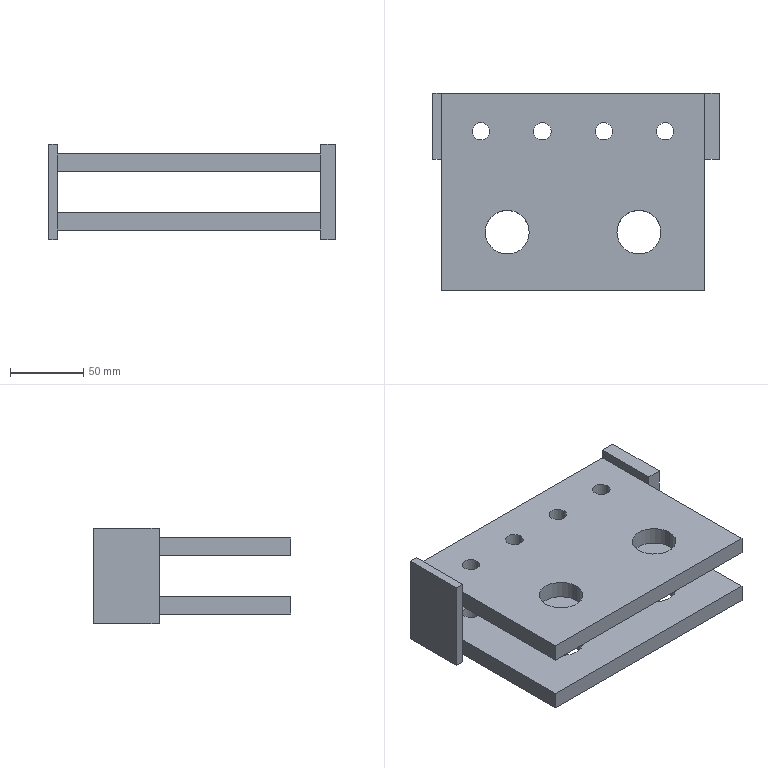Part | STEP file | Counterweight connecting plate_default<machining> | 4 solids | 48 faces | box 196 x 135 x 65 mm | volume 585213 mm3 | plane 24 | cylinder 24 | commonest cylinder face diameters 12 x16 30 x8